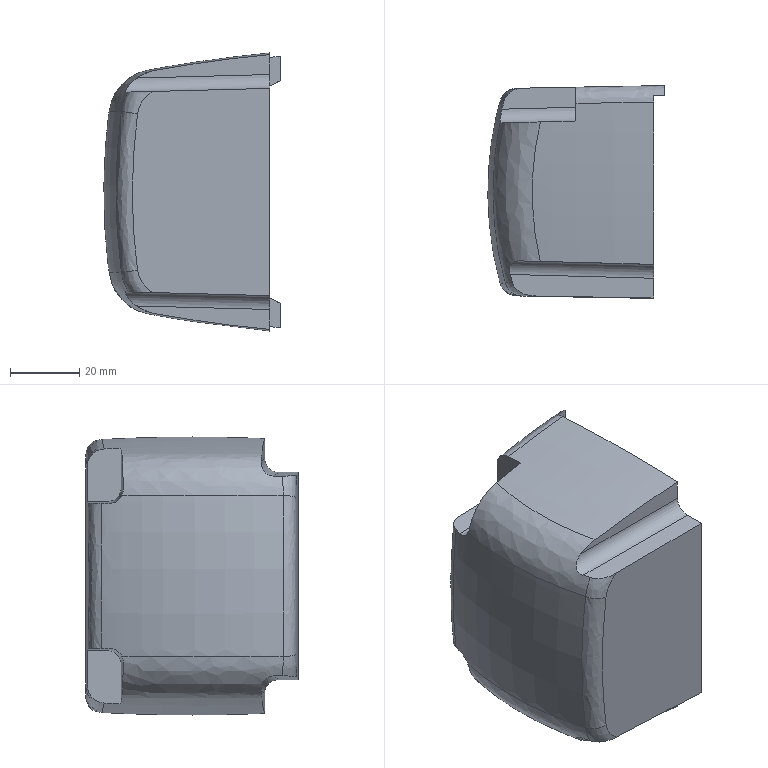Part | STEP file | ASND-0110-IRB120_3-58_IRC5_Link5_rev0 | 1 solid | 34 faces | box 51 x 61.424 x 80.382 mm | volume 189880 mm3 | plane 17 | spline 8 | cylinder 6 | other 3 | commonest cylinder face diameters 8 x4 71 x2